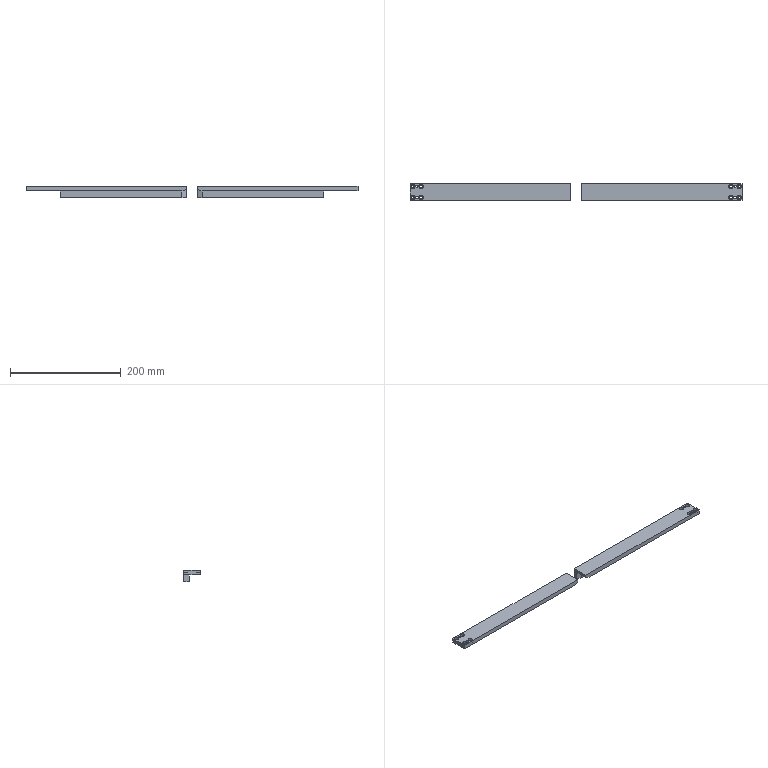NC program | NX | posted with a generic post | part box 600 x 30 x 20 mm
Lines 2349 to 2978 of 2978:
(ZLEVEL_PROFILE_COPY_1_COPY_COPY_COPY_COPY_2_COPY , TOOL : D6A45)
N4654 T02 M6
N4656 G54
N4658 G17 G0 G90 X-123.561 Y11.149 S7000 M3
N4660 G43 Z30. H2
N4662 Z-1.
N4664 G94 G1 X-124.48 Y12.741 F1000.
N4666 G3 X-125. Y13.041 R0.6
N4668 X-128.041 Y10. R3.041
N4670 X-125. Y13.041 R-3.041
N4672 X-125.52 Y12.741 R0.6
N4674 G1 X-126.439 Y11.149
N4676 G0 Z30.
N4678 X-138.561
N4680 Z-1.
N4682 G1 X-139.48 Y12.741
N4684 G3 X-140. Y13.041 R0.6
N4686 X-143.041 Y10. R3.041
N4688 X-140. Y13.041 R-3.041
N4690 X-140.52 Y12.741 R0.6
N4692 G1 X-141.439 Y11.149
N4694 G0 Z30.
N4696 X-133.541 Y-9.5
N4698 Z1.
N4700 G1 Z-1.
N4702 Y-10.5
N4704 G3 X-132.5 Y-11.541 R1.041
N4706 X-131.459 Y-10.5 R1.041
N4708 G1 Y-9.5
N4710 G3 X-132.5 Y-8.459 R1.041
N4712 X-133.541 Y-9.5 R1.041
N4714 X-133.241 Y-10.02 R0.6
N4716 G0 Z30.
N4718 X-126.439 Y-11.149
N4720 Z-1.
N4722 G1 X-125.52 Y-12.741
N4724 G3 X-125. Y-13.041 R0.6
N4726 X-121.959 Y-10. R3.041
N4728 X-125. Y-13.041 R-3.041
N4730 X-124.48 Y-12.741 R0.6
N4732 G1 X-123.561 Y-11.149
N4734 G0 Z30.
N4736 X-141.439
N4738 Z-1.
N4740 G1 X-140.52 Y-12.741
N4742 G3 X-140. Y-13.041 R0.6
N4744 X-136.959 Y-10. R3.041
N4746 X-140. Y-13.041 R-3.041
N4748 X-139.48 Y-12.741 R0.6
N4750 G1 X-138.561 Y-11.149
N4752 G0 Z30.
N4754 X-132.5 Y11.041
N4756 Z1.
N4758 G1 Z-1.
N4760 G3 X-133.541 Y10. R1.041
N4762 X-132.5 Y11.041 R-1.041
N4764 X-133.02 Y10.741 R0.6
N4766 G0 Z30.
N4768 X-145.92 Y16.95
N4770 Z-1.
N4772 G1 X-145.521 Y16.259
N4774 G3 X-145.001 Y15.959 R0.6
N4776 G1 X145.001
N4778 G2 X145.959 Y15.001 R0.966
N4780 G1 Y-15.001
N4782 G2 X145.001 Y-15.959 R0.966
N4784 G1 X-145.001
N4786 G2 X-145.959 Y-15.001 R0.966
N4788 G1 Y15.001
N4790 G2 X-145.001 Y15.959 R0.966
N4792 G3 X-144.484 Y16.263 R0.6
N4794 G1 X-143.976 Y17.159
N4796 G0 Z30.
N4798 M5
(COMPTOOL10_COPY , TOOL : D3)
N4800 T20 M6
N4802 G54
N4804 G17 G0 G90 X-132.352 Y9.977 S7000 M3
N4806 G43 Z30. H20
N4808 Z-0.5
N4810 G94 G1 Z-1. F1000.
N4812 G41 X-132.108 Y9.939 D20
N4814 G3 X-132.119 Y10.239 R0.3
N4816 G1 X-132.122 Y10.243 F850.
N4818 G3 X-132.119 Y9.761 R-0.45
N4820 X-132.119 Y10.239 R0.45
N4822 G1 X-132.184 Y10.312 Z-1.046
N4824 X-132.243 Y10.361 Z-1.083
N4826 X-132.293 Y10.391 Z-1.111
N4828 X-132.383 Y10.426 Z-1.157
N4830 X-132.429 Y10.437 Z-1.179
N4832 X-132.458 Y10.439 Z-1.194
N4834 X-132.516 Y10.442 Z-1.222
N4836 X-132.609 Y10.429 Z-1.266
N4838 X-132.653 Y10.415 Z-1.289
N4840 X-132.681 Y10.404 Z-1.304
N4842 X-132.735 Y10.375 Z-1.333
N4844 X-132.811 Y10.316 Z-1.378
N4846 X-132.86 Y10.258 Z-1.416
N4848 X-132.891 Y10.207 Z-1.444
N4850 X-132.926 Y10.118 Z-1.49
N4852 X-132.936 Y10.072 Z-1.512
N4854 X-132.939 Y10.043 Z-1.527
N4856 X-132.942 Y9.984 Z-1.556
N4858 X-132.929 Y9.891 Z-1.6
N4860 X-132.915 Y9.847 Z-1.622
N4862 X-132.904 Y9.819 Z-1.637
N4864 X-132.875 Y9.765 Z-1.667
N4866 X-132.816 Y9.689 Z-1.712
N4868 X-132.758 Y9.64 Z-1.749
N4870 X-132.707 Y9.609 Z-1.778
N4872 X-132.62 Y9.575 Z-1.822
N4874 X-132.576 Y9.563 Z-1.844
N4876 X-132.545 Y9.56 Z-1.859
N4878 X-132.484 Y9.558 Z-1.889
N4880 X-132.425 Y9.563 Z-1.917
N4882 X-132.369 Y9.578 Z-1.944
N4884 X-132.315 Y9.598 Z-1.972
N4886 X-132.261 Y9.619 Z-2.
N4888 G3 X-132.119 Y9.761 R0.45
N4890 X-132.119 Y10.239 R0.45
N4892 G1 X-132.184 Y10.312 Z-2.046
N4894 X-132.243 Y10.361 Z-2.083
N4896 X-132.293 Y10.391 Z-2.111
N4898 X-132.383 Y10.426 Z-2.157
N4900 X-132.429 Y10.437 Z-2.179
N4902 X-132.458 Y10.439 Z-2.194
N4904 X-132.516 Y10.442 Z-2.222
N4906 X-132.609 Y10.429 Z-2.266
N4908 X-132.653 Y10.415 Z-2.289
N4910 X-132.681 Y10.404 Z-2.304
N4912 X-132.735 Y10.375 Z-2.333
N4914 X-132.811 Y10.316 Z-2.378
N4916 X-132.86 Y10.258 Z-2.416
N4918 X-132.891 Y10.207 Z-2.444
N4920 X-132.926 Y10.118 Z-2.49
N4922 X-132.936 Y10.072 Z-2.512
N4924 X-132.939 Y10.043 Z-2.527
N4926 X-132.942 Y9.984 Z-2.556
N4928 X-132.929 Y9.891 Z-2.6
N4930 X-132.915 Y9.847 Z-2.622
N4932 X-132.904 Y9.819 Z-2.637
N4934 X-132.875 Y9.765 Z-2.667
N4936 X-132.816 Y9.689 Z-2.712
N4938 X-132.758 Y9.64 Z-2.749
N4940 X-132.707 Y9.609 Z-2.778
N4942 X-132.62 Y9.575 Z-2.822
N4944 X-132.576 Y9.563 Z-2.844
N4946 X-132.545 Y9.56 Z-2.859
N4948 X-132.484 Y9.558 Z-2.889
N4950 X-132.425 Y9.563 Z-2.917
N4952 X-132.369 Y9.578 Z-2.944
N4954 X-132.315 Y9.598 Z-2.972
N4956 X-132.261 Y9.619 Z-3.
N4958 G3 X-132.119 Y9.761 R0.45
N4960 X-132.119 Y10.239 R0.45
N4962 G1 X-132.184 Y10.312 Z-3.046
N4964 X-132.243 Y10.361 Z-3.083
N4966 X-132.293 Y10.391 Z-3.111
N4968 X-132.383 Y10.426 Z-3.157
N4970 X-132.428 Y10.437 Z-3.179
N4972 X-132.458 Y10.439 Z-3.194
N4974 X-132.516 Y10.442 Z-3.222
N4976 X-132.609 Y10.429 Z-3.266
N4978 X-132.653 Y10.415 Z-3.289
N4980 X-132.681 Y10.404 Z-3.304
N4982 X-132.735 Y10.375 Z-3.333
N4984 X-132.811 Y10.316 Z-3.378
N4986 X-132.86 Y10.258 Z-3.416
N4988 X-132.891 Y10.207 Z-3.444
N4990 X-132.926 Y10.118 Z-3.49
N4992 X-132.936 Y10.072 Z-3.512
N4994 X-132.939 Y10.043 Z-3.527
N4996 X-132.942 Y9.984 Z-3.556
N4998 X-132.929 Y9.891 Z-3.6
N5000 X-132.915 Y9.847 Z-3.622
N5002 X-132.904 Y9.819 Z-3.637
N5004 X-132.875 Y9.765 Z-3.667
N5006 X-132.816 Y9.689 Z-3.712
N5008 X-132.758 Y9.64 Z-3.749
N5010 X-132.707 Y9.609 Z-3.778
N5012 X-132.62 Y9.575 Z-3.822
N5014 X-132.576 Y9.563 Z-3.844
N5016 X-132.545 Y9.56 Z-3.859
N5018 X-132.484 Y9.558 Z-3.889
N5020 X-132.425 Y9.563 Z-3.917
N5022 X-132.369 Y9.578 Z-3.944
N5024 X-132.315 Y9.598 Z-3.972
N5026 X-132.261 Y9.619 Z-4.
N5028 G3 X-132.119 Y9.761 R0.45
N5030 X-132.119 Y10.239 R0.45
N5032 G1 X-132.184 Y10.312 Z-4.046
N5034 X-132.243 Y10.361 Z-4.083
N5036 X-132.293 Y10.391 Z-4.111
N5038 X-132.383 Y10.426 Z-4.157
N5040 X-132.428 Y10.436 Z-4.179
N5042 X-132.458 Y10.439 Z-4.194
N5044 X-132.516 Y10.442 Z-4.222
N5046 X-132.609 Y10.429 Z-4.266
N5048 X-132.653 Y10.415 Z-4.289
N5050 X-132.681 Y10.404 Z-4.304
N5052 X-132.735 Y10.375 Z-4.333
N5054 X-132.811 Y10.316 Z-4.378
N5056 X-132.86 Y10.258 Z-4.416
N5058 X-132.891 Y10.207 Z-4.444
N5060 X-132.926 Y10.118 Z-4.49
N5062 X-132.936 Y10.072 Z-4.512
N5064 X-132.939 Y10.043 Z-4.527
N5066 X-132.942 Y9.984 Z-4.556
N5068 X-132.929 Y9.891 Z-4.6
N5070 X-132.915 Y9.847 Z-4.622
N5072 X-132.904 Y9.819 Z-4.637
N5074 X-132.875 Y9.765 Z-4.667
N5076 X-132.816 Y9.689 Z-4.712
N5078 X-132.758 Y9.64 Z-4.749
N5080 X-132.707 Y9.609 Z-4.778
N5082 X-132.62 Y9.575 Z-4.822
N5084 X-132.576 Y9.563 Z-4.844
N5086 X-132.545 Y9.56 Z-4.859
N5088 X-132.484 Y9.558 Z-4.889
N5090 X-132.425 Y9.563 Z-4.917
N5092 X-132.369 Y9.578 Z-4.944
N5094 X-132.315 Y9.598 Z-4.972
N5096 X-132.261 Y9.619 Z-5.
N5098 G3 X-132.119 Y9.761 R0.45
N5100 X-132.119 Y10.239 R0.45
N5102 G1 X-132.184 Y10.312 Z-5.046
N5104 X-132.243 Y10.361 Z-5.083
N5106 X-132.293 Y10.391 Z-5.111
N5108 X-132.383 Y10.426 Z-5.157
N5110 X-132.428 Y10.436 Z-5.179
N5112 X-132.458 Y10.439 Z-5.194
N5114 X-132.516 Y10.442 Z-5.222
N5116 X-132.609 Y10.429 Z-5.266
N5118 X-132.653 Y10.415 Z-5.289
N5120 X-132.681 Y10.404 Z-5.304
N5122 X-132.735 Y10.375 Z-5.333
N5124 X-132.811 Y10.316 Z-5.378
N5126 X-132.86 Y10.258 Z-5.416
N5128 X-132.891 Y10.207 Z-5.444
N5130 X-132.926 Y10.118 Z-5.49
N5132 X-132.936 Y10.072 Z-5.512
N5134 X-132.939 Y10.043 Z-5.527
N5136 X-132.942 Y9.984 Z-5.556
N5138 X-132.929 Y9.891 Z-5.6
N5140 X-132.915 Y9.847 Z-5.622
N5142 X-132.904 Y9.819 Z-5.637
N5144 X-132.875 Y9.765 Z-5.667
N5146 X-132.816 Y9.689 Z-5.712
N5148 X-132.758 Y9.64 Z-5.749
N5150 X-132.707 Y9.609 Z-5.778
N5152 X-132.62 Y9.575 Z-5.822
N5154 X-132.576 Y9.563 Z-5.844
N5156 X-132.545 Y9.56 Z-5.859
N5158 X-132.484 Y9.558 Z-5.889
N5160 X-132.425 Y9.563 Z-5.917
N5162 X-132.369 Y9.578 Z-5.944
N5164 X-132.315 Y9.598 Z-5.972
N5166 X-132.261 Y9.619 Z-6.
N5168 G3 X-132.119 Y9.761 R0.45
N5170 X-132.119 Y10.239 R0.45
N5172 G1 X-132.184 Y10.312 Z-6.046
N5174 X-132.243 Y10.361 Z-6.083
N5176 X-132.293 Y10.391 Z-6.111
N5178 X-132.383 Y10.426 Z-6.157
N5180 X-132.428 Y10.436 Z-6.179
N5182 X-132.458 Y10.439 Z-6.194
N5184 X-132.516 Y10.442 Z-6.222
N5186 X-132.609 Y10.429 Z-6.266
N5188 X-132.653 Y10.415 Z-6.289
N5190 X-132.681 Y10.404 Z-6.304
N5192 X-132.735 Y10.374 Z-6.333
N5194 X-132.811 Y10.316 Z-6.378
N5196 X-132.86 Y10.258 Z-6.416
N5198 X-132.891 Y10.207 Z-6.444
N5200 X-132.926 Y10.118 Z-6.49
N5202 X-132.936 Y10.072 Z-6.512
N5204 X-132.939 Y10.043 Z-6.527
N5206 X-132.942 Y9.984 Z-6.556
N5208 X-132.929 Y9.891 Z-6.6
N5210 X-132.915 Y9.847 Z-6.622
N5212 X-132.904 Y9.819 Z-6.637
N5214 X-132.874 Y9.765 Z-6.667
N5216 X-132.816 Y9.689 Z-6.712
N5218 X-132.758 Y9.64 Z-6.749
N5220 X-132.707 Y9.609 Z-6.778
N5222 X-132.62 Y9.575 Z-6.822
N5224 X-132.576 Y9.563 Z-6.844
N5226 X-132.545 Y9.56 Z-6.859
N5228 X-132.484 Y9.558 Z-6.889
N5230 X-132.425 Y9.563 Z-6.917
N5232 X-132.369 Y9.578 Z-6.944
N5234 X-132.315 Y9.599 Z-6.972
N5236 X-132.261 Y9.619 Z-7.
N5238 G3 X-132.119 Y9.761 R0.45
N5240 X-132.119 Y10.239 R0.45
N5242 G1 X-132.184 Y10.312 Z-7.046
N5244 X-132.243 Y10.36 Z-7.083
N5246 X-132.293 Y10.391 Z-7.111
N5248 X-132.383 Y10.426 Z-7.157
N5250 X-132.428 Y10.436 Z-7.179
N5252 X-132.458 Y10.439 Z-7.194
N5254 X-132.516 Y10.442 Z-7.222
N5256 X-132.609 Y10.429 Z-7.266
N5258 X-132.653 Y10.415 Z-7.289
N5260 X-132.681 Y10.404 Z-7.303
N5262 X-132.735 Y10.374 Z-7.333
N5264 X-132.811 Y10.316 Z-7.378
N5266 X-132.86 Y10.258 Z-7.415
N5268 X-132.891 Y10.207 Z-7.444
N5270 X-132.926 Y10.118 Z-7.49
N5272 X-132.936 Y10.073 Z-7.512
N5274 X-132.939 Y10.043 Z-7.527
N5276 X-132.942 Y9.984 Z-7.556
N5278 X-132.929 Y9.891 Z-7.6
N5280 X-132.915 Y9.847 Z-7.622
N5282 X-132.904 Y9.819 Z-7.637
N5284 X-132.874 Y9.765 Z-7.667
N5286 X-132.816 Y9.689 Z-7.712
N5288 X-132.758 Y9.64 Z-7.749
N5290 X-132.707 Y9.609 Z-7.778
N5292 X-132.62 Y9.575 Z-7.822
N5294 X-132.576 Y9.563 Z-7.844
N5296 X-132.545 Y9.561 Z-7.859
N5298 X-132.484 Y9.558 Z-7.889
N5300 X-132.425 Y9.563 Z-7.917
N5302 X-132.369 Y9.578 Z-7.944
N5304 X-132.315 Y9.599 Z-7.972
N5306 X-132.261 Y9.619 Z-8.
N5308 G3 X-132.119 Y9.761 R0.45
N5310 X-132.122 Y10.243 R0.45
N5312 X-132.261 Y9.619 R-0.45
N5314 X-132.12 Y9.884 R0.3
N5316 G40
N5318 G1 X-132.357 Y9.956
N5320 Z-7.5
N5322 G0 Z30.
N5324 X-132.444 Y-10.381
N5326 Z-0.5
N5328 G1 Z-1. F1000.
N5330 G41 X-132.35 Y-10.346
N5332 X-132.2 Y-10.26
N5334 G3 X-132.05 Y-10. R0.3
N5336 G1 Y-9.5 F850.
N5338 G3 X-132.5 Y-9.05 R0.45
N5340 X-132.95 Y-9.5 R0.45
N5342 G1 Y-10.5
N5344 G3 X-132.5 Y-10.95 R0.45
N5346 X-132.05 Y-10.5 R0.45
N5348 G1 Y-10.
N5350 Y-9.638 Z-1.1
N5352 X-132.054 Y-9.517 Z-1.133
N5354 X-132.068 Y-9.406 Z-1.164
N5356 X-132.091 Y-9.331 Z-1.187
N5358 X-132.111 Y-9.289 Z-1.2
N5360 X-132.17 Y-9.206 Z-1.228
N5362 X-132.204 Y-9.171 Z-1.242
N5364 X-132.274 Y-9.12 Z-1.267
N5366 X-132.363 Y-9.08 Z-1.294
N5368 X-132.408 Y-9.066 Z-1.307
N5370 X-132.439 Y-9.062 Z-1.316
N5372 X-132.5 Y-9.056 Z-1.333
N5374 X-132.593 Y-9.066 Z-1.359
N5376 X-132.668 Y-9.09 Z-1.381
N5378 X-132.726 Y-9.12 Z-1.4
N5380 X-132.804 Y-9.178 Z-1.427
N5382 X-132.856 Y-9.237 Z-1.449
N5384 X-132.889 Y-9.289 Z-1.467
N5386 X-132.916 Y-9.35 Z-1.485
N5388 X-132.926 Y-9.382 Z-1.495
N5390 X-132.936 Y-9.426 Z-1.508
N5392 X-132.946 Y-9.517 Z-1.533
N5394 X-132.95 Y-9.638 Z-1.567
N5396 Y-10.362 Z-1.767
N5398 X-132.946 Y-10.483 Z-1.8
N5400 X-132.932 Y-10.594 Z-1.831
N5402 X-132.909 Y-10.669 Z-1.853
N5404 X-132.889 Y-10.711 Z-1.867
N5406 X-132.831 Y-10.793 Z-1.894
N5408 X-132.798 Y-10.828 Z-1.908
N5410 X-132.775 Y-10.846 Z-1.916
N5412 X-132.726 Y-10.88 Z-1.933
N5414 X-132.673 Y-10.909 Z-1.95
N5416 X-132.616 Y-10.926 Z-1.967
N5418 X-132.558 Y-10.938 Z-1.983
N5420 X-132.5 Y-10.95 Z-2.
N5422 G3 X-132.05 Y-10.5 R0.45
N5424 G1 Y-10.
N5426 Y-9.638 Z-2.1
N5428 X-132.054 Y-9.517 Z-2.133
N5430 X-132.068 Y-9.406 Z-2.164
N5432 X-132.091 Y-9.331 Z-2.187
N5434 X-132.111 Y-9.289 Z-2.2
N5436 X-132.17 Y-9.206 Z-2.228
N5438 X-132.204 Y-9.171 Z-2.242
N5440 X-132.274 Y-9.12 Z-2.267
N5442 X-132.363 Y-9.08 Z-2.294
N5444 X-132.408 Y-9.066 Z-2.307
N5446 X-132.439 Y-9.062 Z-2.316
N5448 X-132.5 Y-9.056 Z-2.333
N5450 X-132.593 Y-9.066 Z-2.359
N5452 X-132.668 Y-9.09 Z-2.381
N5454 X-132.726 Y-9.12 Z-2.4
N5456 X-132.804 Y-9.178 Z-2.427
N5458 X-132.856 Y-9.237 Z-2.449
N5460 X-132.889 Y-9.289 Z-2.467
N5462 X-132.916 Y-9.35 Z-2.485
N5464 X-132.926 Y-9.382 Z-2.495
N5466 X-132.936 Y-9.426 Z-2.508
N5468 X-132.946 Y-9.517 Z-2.533
N5470 X-132.95 Y-9.638 Z-2.567
N5472 Y-10.362 Z-2.767
N5474 X-132.946 Y-10.483 Z-2.8
N5476 X-132.932 Y-10.594 Z-2.831
N5478 X-132.909 Y-10.669 Z-2.853
N5480 X-132.889 Y-10.711 Z-2.867
N5482 X-132.831 Y-10.793 Z-2.894
N5484 X-132.798 Y-10.827 Z-2.908
N5486 X-132.775 Y-10.846 Z-2.916
N5488 X-132.726 Y-10.88 Z-2.933
N5490 X-132.673 Y-10.909 Z-2.95
N5492 X-132.616 Y-10.926 Z-2.967
N5494 X-132.558 Y-10.938 Z-2.983
N5496 X-132.5 Y-10.95 Z-3.
N5498 G3 X-132.05 Y-10.5 R0.45
N5500 G1 Y-10.
N5502 Y-9.638 Z-3.1
N5504 X-132.054 Y-9.517 Z-3.133
N5506 X-132.068 Y-9.406 Z-3.164
N5508 X-132.091 Y-9.331 Z-3.187
N5510 X-132.111 Y-9.289 Z-3.2
N5512 X-132.17 Y-9.206 Z-3.228
N5514 X-132.204 Y-9.171 Z-3.242
N5516 X-132.274 Y-9.12 Z-3.267
N5518 X-132.363 Y-9.08 Z-3.294
N5520 X-132.408 Y-9.066 Z-3.307
N5522 X-132.439 Y-9.062 Z-3.316
N5524 X-132.5 Y-9.056 Z-3.333
N5526 X-132.593 Y-9.066 Z-3.359
N5528 X-132.668 Y-9.09 Z-3.381
N5530 X-132.726 Y-9.12 Z-3.4
N5532 X-132.804 Y-9.178 Z-3.427
N5534 X-132.856 Y-9.237 Z-3.449
N5536 X-132.889 Y-9.289 Z-3.467
N5538 X-132.916 Y-9.35 Z-3.485
N5540 X-132.926 Y-9.382 Z-3.495
N5542 X-132.936 Y-9.426 Z-3.508
N5544 X-132.946 Y-9.517 Z-3.533
N5546 X-132.95 Y-9.638 Z-3.567
N5548 Y-10.362 Z-3.767
N5550 X-132.946 Y-10.483 Z-3.8
N5552 X-132.932 Y-10.594 Z-3.831
N5554 X-132.909 Y-10.669 Z-3.853
N5556 X-132.888 Y-10.711 Z-3.867
N5558 X-132.832 Y-10.793 Z-3.894
N5560 X-132.798 Y-10.827 Z-3.908
N5562 X-132.775 Y-10.846 Z-3.916
N5564 X-132.726 Y-10.88 Z-3.933
N5566 X-132.673 Y-10.909 Z-3.95
N5568 X-132.616 Y-10.926 Z-3.967
N5570 X-132.558 Y-10.938 Z-3.983
N5572 X-132.5 Y-10.95 Z-4.
N5574 G3 X-132.05 Y-10.5 R0.45
N5576 G1 Y-10.
N5578 Y-9.638 Z-4.1
N5580 X-132.054 Y-9.517 Z-4.133
N5582 X-132.068 Y-9.406 Z-4.164
N5584 X-132.091 Y-9.331 Z-4.187
N5586 X-132.112 Y-9.289 Z-4.2
N5588 X-132.17 Y-9.206 Z-4.228
N5590 X-132.204 Y-9.172 Z-4.242
N5592 X-132.274 Y-9.12 Z-4.267
N5594 X-132.363 Y-9.08 Z-4.294
N5596 X-132.408 Y-9.066 Z-4.307
N5598 X-132.439 Y-9.062 Z-4.316
N5600 X-132.5 Y-9.056 Z-4.333
N5602 X-132.593 Y-9.066 Z-4.359
N5604 X-132.668 Y-9.09 Z-4.381
N5606 X-132.726 Y-9.12 Z-4.4
N5608 X-132.804 Y-9.178 Z-4.427
N5610 X-132.856 Y-9.237 Z-4.449
N5612 X-132.888 Y-9.289 Z-4.467
N5614 X-132.916 Y-9.35 Z-4.485
N5616 X-132.926 Y-9.381 Z-4.495
N5618 X-132.936 Y-9.426 Z-4.508
N5620 X-132.946 Y-9.517 Z-4.533
N5622 X-132.95 Y-9.638 Z-4.567
N5624 Y-10.362 Z-4.767
N5626 X-132.946 Y-10.483 Z-4.8
N5628 X-132.932 Y-10.594 Z-4.831
N5630 X-132.909 Y-10.669 Z-4.853
N5632 X-132.888 Y-10.711 Z-4.867
N5634 X-132.832 Y-10.793 Z-4.894
N5636 X-132.798 Y-10.827 Z-4.908
N5638 X-132.775 Y-10.846 Z-4.916
N5640 X-132.726 Y-10.88 Z-4.933
N5642 X-132.673 Y-10.909 Z-4.95
N5644 X-132.616 Y-10.926 Z-4.967
N5646 X-132.558 Y-10.938 Z-4.983
N5648 X-132.5 Y-10.95 Z-5.
N5650 G3 X-132.05 Y-10.5 R0.45
N5652 G1 Y-10.
N5654 Y-9.638 Z-5.1
N5656 X-132.054 Y-9.517 Z-5.133
N5658 X-132.068 Y-9.406 Z-5.164
N5660 X-132.091 Y-9.331 Z-5.187
N5662 X-132.112 Y-9.289 Z-5.2
N5664 X-132.17 Y-9.206 Z-5.228
N5666 X-132.204 Y-9.172 Z-5.242
N5668 X-132.227 Y-9.154 Z-5.25
N5670 X-132.274 Y-9.12 Z-5.267
N5672 X-132.363 Y-9.08 Z-5.294
N5674 X-132.408 Y-9.066 Z-5.307
N5676 X-132.439 Y-9.062 Z-5.316
N5678 X-132.5 Y-9.056 Z-5.333
N5680 X-132.593 Y-9.066 Z-5.359
N5682 X-132.667 Y-9.09 Z-5.381
N5684 X-132.726 Y-9.12 Z-5.4
N5686 X-132.804 Y-9.178 Z-5.427
N5688 X-132.856 Y-9.237 Z-5.449
N5690 X-132.888 Y-9.289 Z-5.467
N5692 X-132.916 Y-9.35 Z-5.485
N5694 X-132.926 Y-9.381 Z-5.495
N5696 X-132.936 Y-9.426 Z-5.508
N5698 X-132.946 Y-9.517 Z-5.533
N5700 X-132.95 Y-9.638 Z-5.567
N5702 Y-10.362 Z-5.767
N5704 X-132.946 Y-10.483 Z-5.8
N5706 X-132.932 Y-10.594 Z-5.831
N5708 X-132.911 Y-10.67 Z-5.853
N5710 X-132.888 Y-10.711 Z-5.867
N5712 X-132.829 Y-10.796 Z-5.895
N5714 X-132.794 Y-10.831 Z-5.909
N5716 X-132.772 Y-10.848 Z-5.917
N5718 X-132.726 Y-10.88 Z-5.933
N5720 X-132.673 Y-10.909 Z-5.95
N5722 X-132.616 Y-10.926 Z-5.967
N5724 X-132.558 Y-10.938 Z-5.983
N5726 X-132.5 Y-10.95 Z-6.
N5728 G3 X-132.05 Y-10.5 R0.45
N5730 G1 Y-10.
N5732 Y-9.638 Z-6.1
N5734 X-132.054 Y-9.517 Z-6.133
N5736 X-132.068 Y-9.406 Z-6.164
N5738 X-132.089 Y-9.33 Z-6.187
N5740 X-132.112 Y-9.289 Z-6.2
N5742 X-132.172 Y-9.203 Z-6.229
N5744 X-132.229 Y-9.15 Z-6.251
N5746 X-132.274 Y-9.12 Z-6.267
N5748 X-132.366 Y-9.078 Z-6.295
N5750 X-132.413 Y-9.065 Z-6.308
N5752 X-132.5 Y-9.056 Z-6.333
N5754 X-132.591 Y-9.067 Z-6.359
N5756 X-132.666 Y-9.089 Z-6.381
N5758 X-132.726 Y-9.12 Z-6.4
N5760 X-132.804 Y-9.178 Z-6.427
N5762 X-132.855 Y-9.237 Z-6.449
N5764 X-132.888 Y-9.289 Z-6.467
N5766 X-132.916 Y-9.35 Z-6.485
N5768 X-132.926 Y-9.381 Z-6.495
N5770 X-132.936 Y-9.426 Z-6.508
N5772 X-132.946 Y-9.517 Z-6.533
N5774 X-132.95 Y-9.638 Z-6.567
N5776 Y-10.362 Z-6.767
N5778 X-132.946 Y-10.483 Z-6.8
N5780 X-132.932 Y-10.594 Z-6.831
N5782 X-132.911 Y-10.67 Z-6.853
N5784 X-132.888 Y-10.711 Z-6.867
N5786 X-132.829 Y-10.796 Z-6.895
N5788 X-132.794 Y-10.831 Z-6.909
N5790 X-132.772 Y-10.848 Z-6.917
N5792 X-132.726 Y-10.88 Z-6.933
N5794 X-132.673 Y-10.909 Z-6.95
N5796 X-132.616 Y-10.926 Z-6.967
N5798 X-132.558 Y-10.938 Z-6.983
N5800 X-132.5 Y-10.95 Z-7.
N5802 G3 X-132.05 Y-10.5 R0.45
N5804 G1 Y-10.
N5806 Y-9.638 Z-7.1
N5808 X-132.054 Y-9.517 Z-7.133
N5810 X-132.068 Y-9.406 Z-7.164
N5812 X-132.089 Y-9.33 Z-7.187
N5814 X-132.112 Y-9.289 Z-7.2
N5816 X-132.172 Y-9.203 Z-7.229
N5818 X-132.229 Y-9.15 Z-7.251
N5820 X-132.274 Y-9.12 Z-7.267
N5822 X-132.366 Y-9.079 Z-7.294
N5824 X-132.413 Y-9.065 Z-7.308
N5826 X-132.5 Y-9.056 Z-7.333
N5828 X-132.591 Y-9.067 Z-7.359
N5830 X-132.666 Y-9.089 Z-7.381
N5832 X-132.726 Y-9.12 Z-7.4
N5834 X-132.804 Y-9.178 Z-7.427
N5836 X-132.855 Y-9.237 Z-7.449
N5838 X-132.888 Y-9.289 Z-7.467
N5840 X-132.916 Y-9.35 Z-7.485
N5842 X-132.926 Y-9.381 Z-7.495
N5844 X-132.936 Y-9.426 Z-7.508
N5846 X-132.946 Y-9.517 Z-7.533
N5848 X-132.95 Y-9.638 Z-7.567
N5850 Y-10.362 Z-7.767
N5852 X-132.946 Y-10.483 Z-7.8
N5854 X-132.933 Y-10.595 Z-7.831
N5856 X-132.911 Y-10.67 Z-7.853
N5858 X-132.888 Y-10.711 Z-7.867
N5860 X-132.829 Y-10.795 Z-7.895
N5862 X-132.794 Y-10.831 Z-7.909
N5864 X-132.772 Y-10.848 Z-7.917
N5866 X-132.726 Y-10.88 Z-7.933
N5868 X-132.673 Y-10.909 Z-7.95
N5870 X-132.616 Y-10.926 Z-7.967
N5872 X-132.558 Y-10.938 Z-7.983
N5874 X-132.5 Y-10.95 Z-8.
N5876 G3 X-132.05 Y-10.5 R0.45
N5878 G1 Y-9.5
N5880 G3 X-132.5 Y-9.05 R0.45
N5882 X-132.95 Y-9.5 R0.45
N5884 G1 Y-10.5
N5886 G3 X-132.5 Y-10.95 R0.45
N5888 X-132.24 Y-10.8 R0.3
N5890 G40
N5892 G1 X-132.402 Y-10.613
N5894 Z-7.5
N5896 G0 Z30.
N5898 M5
N5900 M2